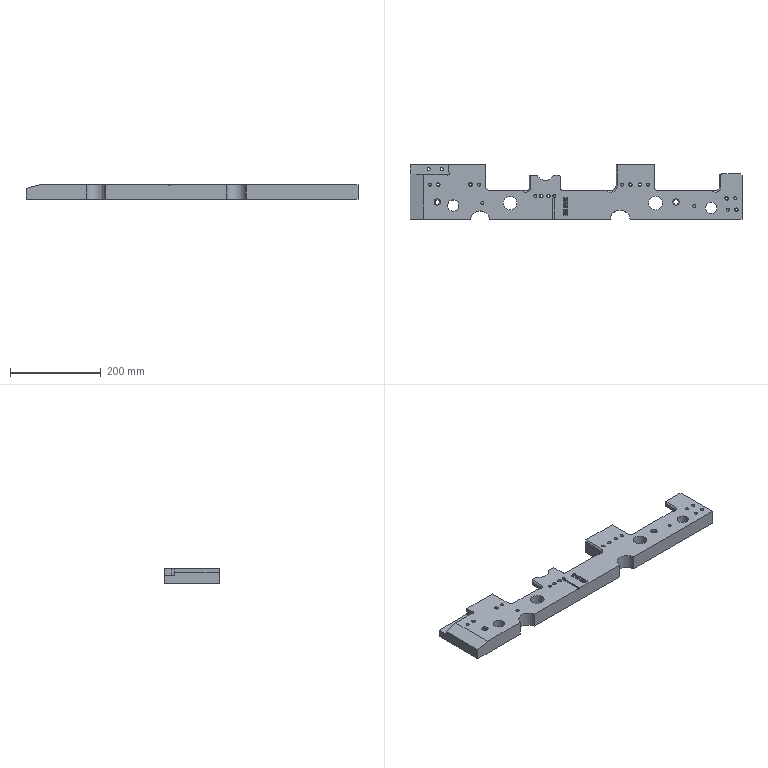Part | STEP file | gslz 2016.10.28-13_id1570_x_t | 1 solid | 216 faces | box 730 x 120 x 32 mm | volume 1766877 mm3 | plane 121 | cylinder 61 | cone 21 | other 13 | commonest cylinder face diameters 6.8 x16 8 x9 6 x8 10 x5 5.2 x4 14 x4